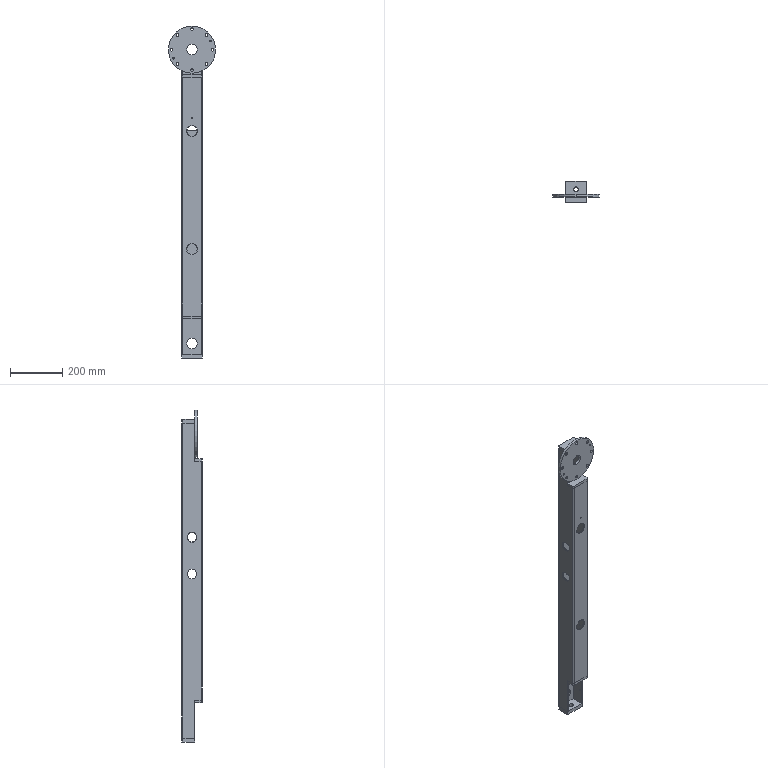Part | SolidWorks | features HoleWzd 9, ICE 8, Cut 3, Fillet 2, Chamfer 1, Extrusion 1, MoveCopyBody 1 | 6 solids | 162 faces | box 180 x 80 x 1265 mm | volume 1908819 mm3 | cylinder 92 | plane 46 | cone 24 | commonest cylinder face diameters 5 x32 11 x16 10 x12 40 x10 35 x8 6 x4